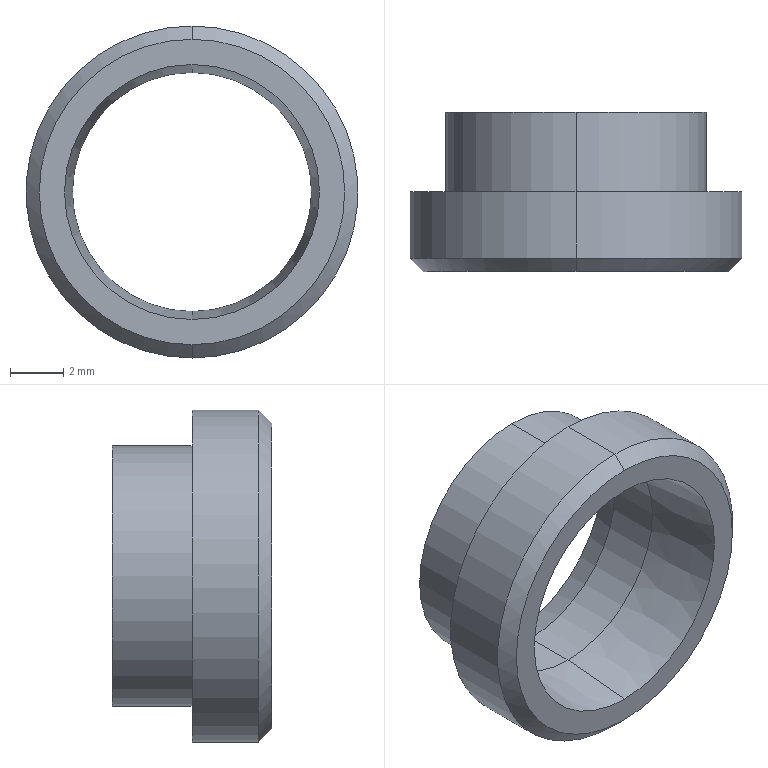Part | SolidWorks | features Chamfer 2, RevCut 1, Revolution 1 | 1 solid | 15 faces | box 12.5 x 6 x 12.5 mm | volume 190.621 mm3 | cone 6 | cylinder 6 | plane 3 | commonest cylinder face diameters 9 x2 9.8 x2 12.5 x2
STEP:
#1=CARTESIAN_POINT('',(0.,5.,-4.5));
#2=VERTEX_POINT('',#1);
#3=CARTESIAN_POINT('',(0.,5.,4.5));
#4=VERTEX_POINT('',#3);
#5=CARTESIAN_POINT('',(0.,5.,0.));
#6=DIRECTION('',(0.,1.,0.));
#7=DIRECTION('',(0.,0.,1.));
#8=AXIS2_PLACEMENT_3D('',#5,#6,#7);
#9=CIRCLE('',#8,4.5);
#10=EDGE_CURVE('',#2,#4,#9,.T.);
#11=ORIENTED_EDGE('',*,*,#10,.F.);
#12=CARTESIAN_POINT('',(0.,6.,-4.8));
#13=VERTEX_POINT('',#12);
#14=CARTESIAN_POINT('',(0.,6.,-4.8));
#15=DIRECTION('',(0.,0.9578,-0.2873));
#16=VECTOR('',#15,1000.);
#17=LINE('',#14,#16);
#18=EDGE_CURVE('',#2,#13,#17,.T.);
#19=ORIENTED_EDGE('',*,*,#18,.T.);
#20=CARTESIAN_POINT('',(0.,6.,4.8));
#21=VERTEX_POINT('',#20);
#22=CARTESIAN_POINT('',(0.,6.,0.));
#23=DIRECTION('',(0.,-1.,0.));
#24=DIRECTION('',(0.,0.,1.));
#25=AXIS2_PLACEMENT_3D('',#22,#23,#24);
#26=CIRCLE('',#25,4.8);
#27=EDGE_CURVE('',#21,#13,#26,.T.);
#28=ORIENTED_EDGE('',*,*,#27,.F.);
#29=CARTESIAN_POINT('',(0.,6.,4.8));
#30=DIRECTION('',(0.,0.9578,0.2873));
#31=VECTOR('',#30,1000.);
#32=LINE('',#29,#31);
#33=EDGE_CURVE('',#4,#21,#32,.T.);
#34=ORIENTED_EDGE('',*,*,#33,.F.);
#35=EDGE_LOOP('',(#11,#19,#28,#34));
#36=FACE_OUTER_BOUND('',#35,.T.);
#37=CARTESIAN_POINT('',(0.,6.,0.));
#38=DIRECTION('',(0.,1.,0.));
#39=DIRECTION('',(0.,0.,1.));
#40=AXIS2_PLACEMENT_3D('',#37,#38,#39);
#41=CONICAL_SURFACE('',#40,4.8,0.2915);
#42=ADVANCED_FACE('',(#36),#41,.F.);
#43=CARTESIAN_POINT('',(0.,0.,-5.75));
#44=VERTEX_POINT('',#43);
#45=CARTESIAN_POINT('',(0.,0.,5.75));
#46=VERTEX_POINT('',#45);
#47=CARTESIAN_POINT('',(0.,0.,0.));
#48=DIRECTION('',(0.,-1.,0.));
#49=DIRECTION('',(0.,0.,-1.));
#50=AXIS2_PLACEMENT_3D('',#47,#48,#49);
#51=CIRCLE('',#50,5.75);
#52=EDGE_CURVE('',#44,#46,#51,.T.);
#53=ORIENTED_EDGE('',*,*,#52,.F.);
#54=CARTESIAN_POINT('',(0.,0.5,-6.25));
#55=VERTEX_POINT('',#54);
#56=CARTESIAN_POINT('',(0.,0.,-5.75));
#57=DIRECTION('',(0.,0.7071,-0.7071));
#58=VECTOR('',#57,1000.);
#59=LINE('',#56,#58);
#60=EDGE_CURVE('',#44,#55,#59,.T.);
#61=ORIENTED_EDGE('',*,*,#60,.T.);
#62=CARTESIAN_POINT('',(0.,0.5,6.25));
#63=VERTEX_POINT('',#62);
#64=CARTESIAN_POINT('',(0.,0.5,0.));
#65=DIRECTION('',(0.,1.,0.));
#66=DIRECTION('',(0.,0.,-1.));
#67=AXIS2_PLACEMENT_3D('',#64,#65,#66);
#68=CIRCLE('',#67,6.25);
#69=EDGE_CURVE('',#63,#55,#68,.T.);
#70=ORIENTED_EDGE('',*,*,#69,.F.);
#71=CARTESIAN_POINT('',(0.,0.,5.75));
#72=DIRECTION('',(0.,0.7071,0.7071));
#73=VECTOR('',#72,1000.);
#74=LINE('',#71,#73);
#75=EDGE_CURVE('',#46,#63,#74,.T.);
#76=ORIENTED_EDGE('',*,*,#75,.F.);
#77=EDGE_LOOP('',(#53,#61,#70,#76));
#78=FACE_OUTER_BOUND('',#77,.T.);
#79=CARTESIAN_POINT('',(0.,0.,0.));
#80=DIRECTION('',(0.,1.,0.));
#81=DIRECTION('',(0.,0.,1.));
#82=AXIS2_PLACEMENT_3D('',#79,#80,#81);
#83=CONICAL_SURFACE('',#82,5.75,0.7854);
#84=ADVANCED_FACE('',(#78),#83,.T.);
#85=CARTESIAN_POINT('',(0.,3.,4.5));
#86=VERTEX_POINT('',#85);
#87=CARTESIAN_POINT('',(0.,3.,-4.5));
#88=VERTEX_POINT('',#87);
#89=CARTESIAN_POINT('',(0.,3.,0.));
#90=DIRECTION('',(0.,-1.,0.));
#91=DIRECTION('',(0.,0.,-1.));
#92=AXIS2_PLACEMENT_3D('',#89,#90,#91);
#93=CIRCLE('',#92,4.5);
#94=EDGE_CURVE('',#86,#88,#93,.T.);
#95=ORIENTED_EDGE('',*,*,#94,.F.);
#96=CARTESIAN_POINT('',(0.,0.,4.8));
#97=VERTEX_POINT('',#96);
#98=CARTESIAN_POINT('',(0.,0.,4.8));
#99=DIRECTION('',(0.,-0.995,0.0995));
#100=VECTOR('',#99,1000.);
#101=LINE('',#98,#100);
#102=EDGE_CURVE('',#86,#97,#101,.T.);
#103=ORIENTED_EDGE('',*,*,#102,.T.);
#104=CARTESIAN_POINT('',(0.,0.,-4.8));
#105=VERTEX_POINT('',#104);
#106=CARTESIAN_POINT('',(0.,0.,0.));
#107=DIRECTION('',(0.,-1.,0.));
#108=DIRECTION('',(0.,0.,-1.));
#109=AXIS2_PLACEMENT_3D('',#106,#107,#108);
#110=CIRCLE('',#109,4.8);
#111=EDGE_CURVE('',#97,#105,#110,.T.);
#112=ORIENTED_EDGE('',*,*,#111,.T.);
#113=CARTESIAN_POINT('',(0.,0.,-4.8));
#114=DIRECTION('',(0.,-0.995,-0.0995));
#115=VECTOR('',#114,1000.);
#116=LINE('',#113,#115);
#117=EDGE_CURVE('',#88,#105,#116,.T.);
#118=ORIENTED_EDGE('',*,*,#117,.F.);
#119=EDGE_LOOP('',(#95,#103,#112,#118));
#120=FACE_OUTER_BOUND('',#119,.T.);
#121=CARTESIAN_POINT('',(0.,0.,0.));
#122=DIRECTION('',(0.,-1.,0.));
#123=DIRECTION('',(0.,0.,-1.));
#124=AXIS2_PLACEMENT_3D('',#121,#122,#123);
#125=CONICAL_SURFACE('',#124,4.8,0.09967);
#126=ADVANCED_FACE('',(#120),#125,.F.);
#127=CARTESIAN_POINT('',(0.,3.,-6.25));
#128=VERTEX_POINT('',#127);
#129=CARTESIAN_POINT('',(0.,3.,6.25));
#130=VERTEX_POINT('',#129);
#131=CARTESIAN_POINT('',(0.,3.,0.));
#132=DIRECTION('',(0.,-1.,0.));
#133=DIRECTION('',(0.,0.,-1.));
#134=AXIS2_PLACEMENT_3D('',#131,#132,#133);
#135=CIRCLE('',#134,6.25);
#136=EDGE_CURVE('',#128,#130,#135,.T.);
#137=ORIENTED_EDGE('',*,*,#136,.T.);
#138=CARTESIAN_POINT('',(0.,0.,6.25));
#139=DIRECTION('',(0.,-1.,0.));
#140=VECTOR('',#139,1000.);
#141=LINE('',#138,#140);
#142=EDGE_CURVE('',#130,#63,#141,.T.);
#143=ORIENTED_EDGE('',*,*,#142,.T.);
#144=ORIENTED_EDGE('',*,*,#69,.T.);
#145=CARTESIAN_POINT('',(0.,0.,-6.25));
#146=DIRECTION('',(0.,-1.,0.));
#147=VECTOR('',#146,1000.);
#148=LINE('',#145,#147);
#149=EDGE_CURVE('',#128,#55,#148,.T.);
#150=ORIENTED_EDGE('',*,*,#149,.F.);
#151=EDGE_LOOP('',(#137,#143,#144,#150));
#152=FACE_OUTER_BOUND('',#151,.T.);
#153=CARTESIAN_POINT('',(0.,0.,0.));
#154=DIRECTION('',(0.,-1.,0.));
#155=DIRECTION('',(0.,0.,-1.));
#156=AXIS2_PLACEMENT_3D('',#153,#154,#155);
#157=CYLINDRICAL_SURFACE('',#156,6.25);
#158=ADVANCED_FACE('',(#152),#157,.T.);
#159=CARTESIAN_POINT('',(0.,6.,-4.9));
#160=VERTEX_POINT('',#159);
#161=CARTESIAN_POINT('',(0.,6.,4.9));
#162=VERTEX_POINT('',#161);
#163=CARTESIAN_POINT('',(0.,6.,0.));
#164=DIRECTION('',(0.,-1.,0.));
#165=DIRECTION('',(0.,0.,-1.));
#166=AXIS2_PLACEMENT_3D('',#163,#164,#165);
#167=CIRCLE('',#166,4.9);
#168=EDGE_CURVE('',#160,#162,#167,.T.);
#169=ORIENTED_EDGE('',*,*,#168,.T.);
#170=CARTESIAN_POINT('',(0.,3.,4.9));
#171=VERTEX_POINT('',#170);
#172=CARTESIAN_POINT('',(0.,0.,4.9));
#173=DIRECTION('',(0.,-1.,0.));
#174=VECTOR('',#173,1000.);
#175=LINE('',#172,#174);
#176=EDGE_CURVE('',#162,#171,#175,.T.);
#177=ORIENTED_EDGE('',*,*,#176,.T.);
#178=CARTESIAN_POINT('',(0.,3.,-4.9));
#179=VERTEX_POINT('',#178);
#180=CARTESIAN_POINT('',(0.,3.,0.));
#181=DIRECTION('',(0.,-1.,0.));
#182=DIRECTION('',(0.,0.,-1.));
#183=AXIS2_PLACEMENT_3D('',#180,#181,#182);
#184=CIRCLE('',#183,4.9);
#185=EDGE_CURVE('',#179,#171,#184,.T.);
#186=ORIENTED_EDGE('',*,*,#185,.F.);
#187=CARTESIAN_POINT('',(0.,0.,-4.9));
#188=DIRECTION('',(0.,-1.,0.));
#189=VECTOR('',#188,1000.);
#190=LINE('',#187,#189);
#191=EDGE_CURVE('',#160,#179,#190,.T.);
#192=ORIENTED_EDGE('',*,*,#191,.F.);
#193=EDGE_LOOP('',(#169,#177,#186,#192));
#194=FACE_OUTER_BOUND('',#193,.T.);
#195=CARTESIAN_POINT('',(0.,0.,0.));
#196=DIRECTION('',(0.,-1.,0.));
#197=DIRECTION('',(0.,0.,-1.));
#198=AXIS2_PLACEMENT_3D('',#195,#196,#197);
#199=CYLINDRICAL_SURFACE('',#198,4.9);
#200=ADVANCED_FACE('',(#194),#199,.T.);
#201=ORIENTED_EDGE('',*,*,#10,.T.);
#202=CARTESIAN_POINT('',(0.,0.,4.5));
#203=DIRECTION('',(0.,-1.,0.));
#204=VECTOR('',#203,1000.);
#205=LINE('',#202,#204);
#206=EDGE_CURVE('',#4,#86,#205,.T.);
#207=ORIENTED_EDGE('',*,*,#206,.T.);
#208=ORIENTED_EDGE('',*,*,#94,.T.);
#209=CARTESIAN_POINT('',(0.,0.,-4.5));
#210=DIRECTION('',(0.,-1.,0.));
#211=VECTOR('',#210,1000.);
#212=LINE('',#209,#211);
#213=EDGE_CURVE('',#2,#88,#212,.T.);
#214=ORIENTED_EDGE('',*,*,#213,.F.);
#215=EDGE_LOOP('',(#201,#207,#208,#214));
#216=FACE_OUTER_BOUND('',#215,.T.);
#217=CARTESIAN_POINT('',(0.,0.,0.));
#218=DIRECTION('',(0.,-1.,0.));
#219=DIRECTION('',(0.,0.,-1.));
#220=AXIS2_PLACEMENT_3D('',#217,#218,#219);
#221=CYLINDRICAL_SURFACE('',#220,4.5);
#222=ADVANCED_FACE('',(#216),#221,.F.);
#223=CARTESIAN_POINT('',(0.,0.,0.));
#224=DIRECTION('',(0.,-1.,0.));
#225=DIRECTION('',(0.,0.,-1.));
#226=AXIS2_PLACEMENT_3D('',#223,#224,#225);
#227=CIRCLE('',#226,5.75);
#228=EDGE_CURVE('',#46,#44,#227,.T.);
#229=ORIENTED_EDGE('',*,*,#228,.T.);
#230=ORIENTED_EDGE('',*,*,#52,.T.);
#231=EDGE_LOOP('',(#229,#230));
#232=FACE_OUTER_BOUND('',#231,.T.);
#233=CARTESIAN_POINT('',(0.,0.,0.));
#234=DIRECTION('',(0.,-1.,0.));
#235=DIRECTION('',(0.,0.,-1.));
#236=AXIS2_PLACEMENT_3D('',#233,#234,#235);
#237=CIRCLE('',#236,4.8);
#238=EDGE_CURVE('',#105,#97,#237,.T.);
#239=ORIENTED_EDGE('',*,*,#238,.F.);
#240=ORIENTED_EDGE('',*,*,#111,.F.);
#241=EDGE_LOOP('',(#239,#240));
#242=FACE_BOUND('',#241,.T.);
#243=CARTESIAN_POINT('',(6.25,0.,0.));
#244=DIRECTION('',(0.,-1.,0.));
#245=DIRECTION('',(0.,0.,-1.));
#246=AXIS2_PLACEMENT_3D('',#243,#244,#245);
#247=PLANE('',#246);
#248=ADVANCED_FACE('',(#232,#242),#247,.T.);
#249=ORIENTED_EDGE('',*,*,#206,.F.);
#250=CARTESIAN_POINT('',(0.,5.,0.));
#251=DIRECTION('',(0.,1.,0.));
#252=DIRECTION('',(0.,0.,1.));
#253=AXIS2_PLACEMENT_3D('',#250,#251,#252);
#254=CIRCLE('',#253,4.5);
#255=EDGE_CURVE('',#4,#2,#254,.T.);
#256=ORIENTED_EDGE('',*,*,#255,.T.);
#257=ORIENTED_EDGE('',*,*,#213,.T.);
#258=CARTESIAN_POINT('',(0.,3.,0.));
#259=DIRECTION('',(0.,-1.,0.));
#260=DIRECTION('',(0.,0.,-1.));
#261=AXIS2_PLACEMENT_3D('',#258,#259,#260);
#262=CIRCLE('',#261,4.5);
#263=EDGE_CURVE('',#88,#86,#262,.T.);
#264=ORIENTED_EDGE('',*,*,#263,.T.);
#265=EDGE_LOOP('',(#249,#256,#257,#264));
#266=FACE_OUTER_BOUND('',#265,.T.);
#267=CARTESIAN_POINT('',(0.,0.,0.));
#268=DIRECTION('',(0.,-1.,0.));
#269=DIRECTION('',(0.,0.,-1.));
#270=AXIS2_PLACEMENT_3D('',#267,#268,#269);
#271=CYLINDRICAL_SURFACE('',#270,4.5);
#272=ADVANCED_FACE('',(#266),#271,.F.);
#273=ORIENTED_EDGE('',*,*,#27,.T.);
#274=CARTESIAN_POINT('',(0.,6.,0.));
#275=DIRECTION('',(0.,-1.,0.));
#276=DIRECTION('',(0.,0.,1.));
#277=AXIS2_PLACEMENT_3D('',#274,#275,#276);
#278=CIRCLE('',#277,4.8);
#279=EDGE_CURVE('',#13,#21,#278,.T.);
#280=ORIENTED_EDGE('',*,*,#279,.T.);
#281=EDGE_LOOP('',(#273,#280));
#282=FACE_BOUND('',#281,.T.);
#283=ORIENTED_EDGE('',*,*,#168,.F.);
#284=CARTESIAN_POINT('',(0.,6.,0.));
#285=DIRECTION('',(0.,-1.,0.));
#286=DIRECTION('',(0.,0.,-1.));
#287=AXIS2_PLACEMENT_3D('',#284,#285,#286);
#288=CIRCLE('',#287,4.9);
#289=EDGE_CURVE('',#162,#160,#288,.T.);
#290=ORIENTED_EDGE('',*,*,#289,.F.);
#291=EDGE_LOOP('',(#283,#290));
#292=FACE_OUTER_BOUND('',#291,.T.);
#293=CARTESIAN_POINT('',(4.5,6.,0.));
#294=DIRECTION('',(0.,1.,0.));
#295=DIRECTION('',(0.,0.,1.));
#296=AXIS2_PLACEMENT_3D('',#293,#294,#295);
#297=PLANE('',#296);
#298=ADVANCED_FACE('',(#282,#292),#297,.T.);
#299=ORIENTED_EDGE('',*,*,#176,.F.);
#300=ORIENTED_EDGE('',*,*,#289,.T.);
#301=ORIENTED_EDGE('',*,*,#191,.T.);
#302=CARTESIAN_POINT('',(0.,3.,0.));
#303=DIRECTION('',(0.,-1.,0.));
#304=DIRECTION('',(0.,0.,-1.));
#305=AXIS2_PLACEMENT_3D('',#302,#303,#304);
#306=CIRCLE('',#305,4.9);
#307=EDGE_CURVE('',#171,#179,#306,.T.);
#308=ORIENTED_EDGE('',*,*,#307,.F.);
#309=EDGE_LOOP('',(#299,#300,#301,#308));
#310=FACE_OUTER_BOUND('',#309,.T.);
#311=CARTESIAN_POINT('',(0.,0.,0.));
#312=DIRECTION('',(0.,-1.,0.));
#313=DIRECTION('',(0.,0.,-1.));
#314=AXIS2_PLACEMENT_3D('',#311,#312,#313);
#315=CYLINDRICAL_SURFACE('',#314,4.9);
#316=ADVANCED_FACE('',(#310),#315,.T.);
#317=ORIENTED_EDGE('',*,*,#185,.T.);
#318=ORIENTED_EDGE('',*,*,#307,.T.);
#319=EDGE_LOOP('',(#317,#318));
#320=FACE_BOUND('',#319,.T.);
#321=ORIENTED_EDGE('',*,*,#136,.F.);
#322=CARTESIAN_POINT('',(0.,3.,0.));
#323=DIRECTION('',(0.,-1.,0.));
#324=DIRECTION('',(0.,0.,-1.));
#325=AXIS2_PLACEMENT_3D('',#322,#323,#324);
#326=CIRCLE('',#325,6.25);
#327=EDGE_CURVE('',#130,#128,#326,.T.);
#328=ORIENTED_EDGE('',*,*,#327,.F.);
#329=EDGE_LOOP('',(#321,#328));
#330=FACE_OUTER_BOUND('',#329,.T.);
#331=CARTESIAN_POINT('',(4.9,3.,0.));
#332=DIRECTION('',(0.,1.,0.));
#333=DIRECTION('',(0.,0.,1.));
#334=AXIS2_PLACEMENT_3D('',#331,#332,#333);
#335=PLANE('',#334);
#336=ADVANCED_FACE('',(#320,#330),#335,.T.);
#337=ORIENTED_EDGE('',*,*,#142,.F.);
#338=ORIENTED_EDGE('',*,*,#327,.T.);
#339=ORIENTED_EDGE('',*,*,#149,.T.);
#340=CARTESIAN_POINT('',(0.,0.5,0.));
#341=DIRECTION('',(0.,1.,0.));
#342=DIRECTION('',(0.,0.,-1.));
#343=AXIS2_PLACEMENT_3D('',#340,#341,#342);
#344=CIRCLE('',#343,6.25);
#345=EDGE_CURVE('',#55,#63,#344,.T.);
#346=ORIENTED_EDGE('',*,*,#345,.T.);
#347=EDGE_LOOP('',(#337,#338,#339,#346));
#348=FACE_OUTER_BOUND('',#347,.T.);
#349=CARTESIAN_POINT('',(0.,0.,0.));
#350=DIRECTION('',(0.,-1.,0.));
#351=DIRECTION('',(0.,0.,-1.));
#352=AXIS2_PLACEMENT_3D('',#349,#350,#351);
#353=CYLINDRICAL_SURFACE('',#352,6.25);
#354=ADVANCED_FACE('',(#348),#353,.T.);
#355=ORIENTED_EDGE('',*,*,#102,.F.);
#356=ORIENTED_EDGE('',*,*,#263,.F.);
#357=ORIENTED_EDGE('',*,*,#117,.T.);
#358=ORIENTED_EDGE('',*,*,#238,.T.);
#359=EDGE_LOOP('',(#355,#356,#357,#358));
#360=FACE_OUTER_BOUND('',#359,.T.);
#361=CARTESIAN_POINT('',(0.,0.,0.));
#362=DIRECTION('',(0.,-1.,0.));
#363=DIRECTION('',(0.,0.,-1.));
#364=AXIS2_PLACEMENT_3D('',#361,#362,#363);
#365=CONICAL_SURFACE('',#364,4.8,0.09967);
#366=ADVANCED_FACE('',(#360),#365,.F.);
#367=ORIENTED_EDGE('',*,*,#60,.F.);
#368=ORIENTED_EDGE('',*,*,#228,.F.);
#369=ORIENTED_EDGE('',*,*,#75,.T.);
#370=ORIENTED_EDGE('',*,*,#345,.F.);
#371=EDGE_LOOP('',(#367,#368,#369,#370));
#372=FACE_OUTER_BOUND('',#371,.T.);
#373=CARTESIAN_POINT('',(0.,0.,0.));
#374=DIRECTION('',(0.,1.,0.));
#375=DIRECTION('',(0.,0.,1.));
#376=AXIS2_PLACEMENT_3D('',#373,#374,#375);
#377=CONICAL_SURFACE('',#376,5.75,0.7854);
#378=ADVANCED_FACE('',(#372),#377,.T.);
#379=ORIENTED_EDGE('',*,*,#18,.F.);
#380=ORIENTED_EDGE('',*,*,#255,.F.);
#381=ORIENTED_EDGE('',*,*,#33,.T.);
#382=ORIENTED_EDGE('',*,*,#279,.F.);
#383=EDGE_LOOP('',(#379,#380,#381,#382));
#384=FACE_OUTER_BOUND('',#383,.T.);
#385=CARTESIAN_POINT('',(0.,6.,0.));
#386=DIRECTION('',(0.,1.,0.));
#387=DIRECTION('',(0.,0.,1.));
#388=AXIS2_PLACEMENT_3D('',#385,#386,#387);
#389=CONICAL_SURFACE('',#388,4.8,0.2915);
#390=ADVANCED_FACE('',(#384),#389,.F.);
#391=CLOSED_SHELL('',(#42,#84,#126,#158,#200,#222,#248,#272,#298,#316,#336,#354,#366,#378,#390));
#392=MANIFOLD_SOLID_BREP('',#391);
#393=CARTESIAN_POINT('',(0.,0.,0.));
#394=DIRECTION('',(0.,0.,1.));
#395=DIRECTION('',(1.,0.,0.));
#396=AXIS2_PLACEMENT_3D('',#393,#394,#395);
#397=(LENGTH_UNIT()NAMED_UNIT(*)SI_UNIT(.MILLI.,.METRE.));
#398=UNCERTAINTY_MEASURE_WITH_UNIT(LENGTH_MEASURE(0.00001),#397,'','');
#399=(NAMED_UNIT(*)PLANE_ANGLE_UNIT()SI_UNIT($,.RADIAN.));
#400=(NAMED_UNIT(*)SI_UNIT($,.STERADIAN.)SOLID_ANGLE_UNIT());
#401=(GEOMETRIC_REPRESENTATION_CONTEXT(3)GLOBAL_UNCERTAINTY_ASSIGNED_CONTEXT((#398))GLOBAL_UNIT_ASSIGNED_CONTEXT((#397,#399,#400))REPRESENTATION_CONTEXT('',''));
#402=ADVANCED_BREP_SHAPE_REPRESENTATION('',(#392,#396),#401);